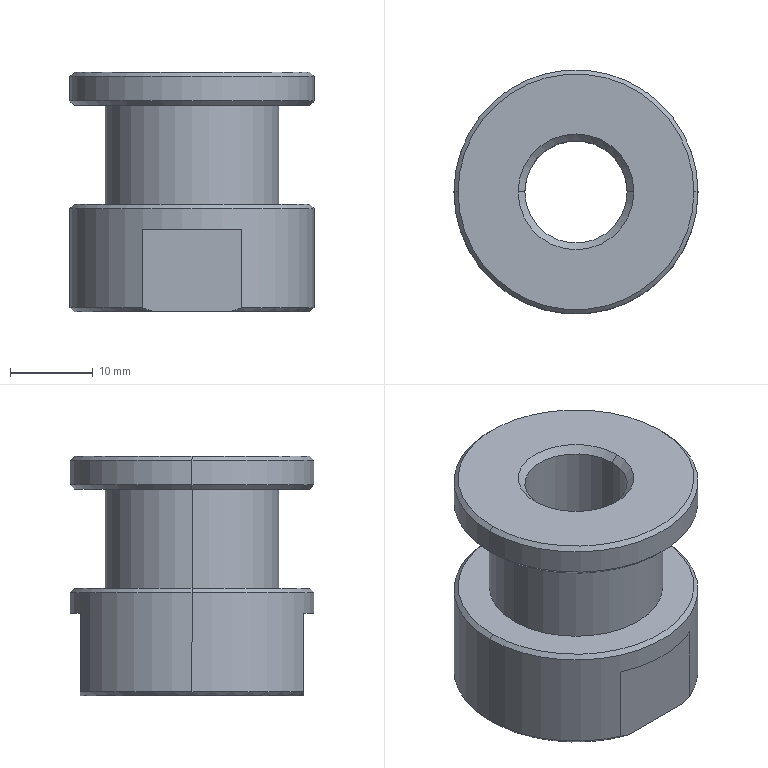Part | SolidWorks | features BaseBody 1 | 1 solid | 28 faces | box 29.5 x 29.5 x 29 mm | volume 12018 mm3 | cone 12 | cylinder 8 | plane 8 | commonest cylinder face diameters 29.5 x4 12.376 x2 21 x2
STEP:
#1=CARTESIAN_POINT('',(-6.188,0.,-28.188));
#2=VERTEX_POINT('',#1);
#3=CARTESIAN_POINT('',(6.188,0.,-28.188));
#4=VERTEX_POINT('',#3);
#5=CARTESIAN_POINT('',(0.,0.,-28.188));
#6=DIRECTION('',(0.,0.,1.));
#7=DIRECTION('',(1.,0.,0.));
#8=AXIS2_PLACEMENT_3D('',#5,#6,#7);
#9=CIRCLE('',#8,6.188);
#10=EDGE_CURVE('',#2,#4,#9,.T.);
#11=ORIENTED_EDGE('',*,*,#10,.F.);
#12=CARTESIAN_POINT('',(-6.188,0.,-0.812));
#13=VERTEX_POINT('',#12);
#14=CARTESIAN_POINT('',(-6.188,0.,-50.));
#15=DIRECTION('',(0.,0.,1.));
#16=VECTOR('',#15,1000.);
#17=LINE('',#14,#16);
#18=EDGE_CURVE('',#2,#13,#17,.T.);
#19=ORIENTED_EDGE('',*,*,#18,.T.);
#20=CARTESIAN_POINT('',(6.188,0.,-0.812));
#21=VERTEX_POINT('',#20);
#22=CARTESIAN_POINT('',(0.,0.,-0.812));
#23=DIRECTION('',(0.,0.,-1.));
#24=DIRECTION('',(1.,0.,0.));
#25=AXIS2_PLACEMENT_3D('',#22,#23,#24);
#26=CIRCLE('',#25,6.188);
#27=EDGE_CURVE('',#21,#13,#26,.T.);
#28=ORIENTED_EDGE('',*,*,#27,.F.);
#29=CARTESIAN_POINT('',(6.188,0.,-50.));
#30=DIRECTION('',(0.,0.,1.));
#31=VECTOR('',#30,1000.);
#32=LINE('',#29,#31);
#33=EDGE_CURVE('',#4,#21,#32,.T.);
#34=ORIENTED_EDGE('',*,*,#33,.F.);
#35=EDGE_LOOP('',(#11,#19,#28,#34));
#36=FACE_OUTER_BOUND('',#35,.T.);
#37=CARTESIAN_POINT('',(0.,0.,-50.));
#38=DIRECTION('',(0.,0.,1.));
#39=DIRECTION('',(1.,0.,0.));
#40=AXIS2_PLACEMENT_3D('',#37,#38,#39);
#41=CYLINDRICAL_SURFACE('',#40,6.188);
#42=ADVANCED_FACE('',(#36),#41,.F.);
#43=ORIENTED_EDGE('',*,*,#27,.T.);
#44=CARTESIAN_POINT('',(-7.,0.,0.));
#45=VERTEX_POINT('',#44);
#46=CARTESIAN_POINT('',(-7.,0.,0.));
#47=DIRECTION('',(-0.7071,0.,0.7071));
#48=VECTOR('',#47,1000.);
#49=LINE('',#46,#48);
#50=EDGE_CURVE('',#13,#45,#49,.T.);
#51=ORIENTED_EDGE('',*,*,#50,.T.);
#52=CARTESIAN_POINT('',(7.,0.,0.));
#53=VERTEX_POINT('',#52);
#54=CARTESIAN_POINT('',(0.,0.,0.));
#55=DIRECTION('',(0.,0.,-1.));
#56=DIRECTION('',(1.,0.,0.));
#57=AXIS2_PLACEMENT_3D('',#54,#55,#56);
#58=CIRCLE('',#57,7.);
#59=EDGE_CURVE('',#53,#45,#58,.T.);
#60=ORIENTED_EDGE('',*,*,#59,.F.);
#61=CARTESIAN_POINT('',(7.,0.,0.));
#62=DIRECTION('',(0.7071,0.,0.7071));
#63=VECTOR('',#62,1000.);
#64=LINE('',#61,#63);
#65=EDGE_CURVE('',#21,#53,#64,.T.);
#66=ORIENTED_EDGE('',*,*,#65,.F.);
#67=EDGE_LOOP('',(#43,#51,#60,#66));
#68=FACE_OUTER_BOUND('',#67,.T.);
#69=CARTESIAN_POINT('',(0.,0.,0.));
#70=DIRECTION('',(0.,0.,1.));
#71=DIRECTION('',(1.,0.,0.));
#72=AXIS2_PLACEMENT_3D('',#69,#70,#71);
#73=CONICAL_SURFACE('',#72,7.,0.7854);
#74=ADVANCED_FACE('',(#68),#73,.F.);
#75=ORIENTED_EDGE('',*,*,#10,.T.);
#76=CARTESIAN_POINT('',(7.,0.,-29.));
#77=VERTEX_POINT('',#76);
#78=CARTESIAN_POINT('',(7.,0.,-29.));
#79=DIRECTION('',(0.7071,0.,-0.7071));
#80=VECTOR('',#79,1000.);
#81=LINE('',#78,#80);
#82=EDGE_CURVE('',#4,#77,#81,.T.);
#83=ORIENTED_EDGE('',*,*,#82,.T.);
#84=CARTESIAN_POINT('',(-7.,0.,-29.));
#85=VERTEX_POINT('',#84);
#86=CARTESIAN_POINT('',(0.,0.,-29.));
#87=DIRECTION('',(0.,0.,1.));
#88=DIRECTION('',(-1.,0.,0.));
#89=AXIS2_PLACEMENT_3D('',#86,#87,#88);
#90=CIRCLE('',#89,7.);
#91=EDGE_CURVE('',#85,#77,#90,.T.);
#92=ORIENTED_EDGE('',*,*,#91,.F.);
#93=CARTESIAN_POINT('',(-7.,0.,-29.));
#94=DIRECTION('',(-0.7071,0.,-0.7071));
#95=VECTOR('',#94,1000.);
#96=LINE('',#93,#95);
#97=EDGE_CURVE('',#2,#85,#96,.T.);
#98=ORIENTED_EDGE('',*,*,#97,.F.);
#99=EDGE_LOOP('',(#75,#83,#92,#98));
#100=FACE_OUTER_BOUND('',#99,.T.);
#101=CARTESIAN_POINT('',(0.,0.,-29.));
#102=DIRECTION('',(0.,0.,-1.));
#103=DIRECTION('',(-1.,0.,0.));
#104=AXIS2_PLACEMENT_3D('',#101,#102,#103);
#105=CONICAL_SURFACE('',#104,7.,0.7854);
#106=ADVANCED_FACE('',(#100),#105,.F.);
#107=CARTESIAN_POINT('',(-14.25,0.,0.));
#108=VERTEX_POINT('',#107);
#109=CARTESIAN_POINT('',(14.25,0.,0.));
#110=VERTEX_POINT('',#109);
#111=CARTESIAN_POINT('',(0.,0.,0.));
#112=DIRECTION('',(0.,0.,-1.));
#113=DIRECTION('',(-1.,0.,0.));
#114=AXIS2_PLACEMENT_3D('',#111,#112,#113);
#115=CIRCLE('',#114,14.25);
#116=EDGE_CURVE('',#108,#110,#115,.T.);
#117=ORIENTED_EDGE('',*,*,#116,.T.);
#118=CARTESIAN_POINT('',(14.75,0.,-0.5));
#119=VERTEX_POINT('',#118);
#120=CARTESIAN_POINT('',(14.75,0.,-0.5));
#121=DIRECTION('',(0.7071,0.,-0.7071));
#122=VECTOR('',#121,1000.);
#123=LINE('',#120,#122);
#124=EDGE_CURVE('',#110,#119,#123,.T.);
#125=ORIENTED_EDGE('',*,*,#124,.T.);
#126=CARTESIAN_POINT('',(-14.75,0.,-0.5));
#127=VERTEX_POINT('',#126);
#128=CARTESIAN_POINT('',(0.,0.,-0.5));
#129=DIRECTION('',(0.,0.,1.));
#130=DIRECTION('',(-1.,0.,0.));
#131=AXIS2_PLACEMENT_3D('',#128,#129,#130);
#132=CIRCLE('',#131,14.75);
#133=EDGE_CURVE('',#119,#127,#132,.T.);
#134=ORIENTED_EDGE('',*,*,#133,.T.);
#135=CARTESIAN_POINT('',(-14.75,0.,-0.5));
#136=DIRECTION('',(-0.7071,0.,-0.7071));
#137=VECTOR('',#136,1000.);
#138=LINE('',#135,#137);
#139=EDGE_CURVE('',#108,#127,#138,.T.);
#140=ORIENTED_EDGE('',*,*,#139,.F.);
#141=EDGE_LOOP('',(#117,#125,#134,#140));
#142=FACE_OUTER_BOUND('',#141,.T.);
#143=CARTESIAN_POINT('',(0.,0.,-0.5));
#144=DIRECTION('',(0.,0.,-1.));
#145=DIRECTION('',(-1.,0.,0.));
#146=AXIS2_PLACEMENT_3D('',#143,#144,#145);
#147=CONICAL_SURFACE('',#146,14.75,0.7854);
#148=ADVANCED_FACE('',(#142),#147,.T.);
#149=CARTESIAN_POINT('',(14.75,0.,-3.5));
#150=VERTEX_POINT('',#149);
#151=CARTESIAN_POINT('',(-14.75,0.,-3.5));
#152=VERTEX_POINT('',#151);
#153=CARTESIAN_POINT('',(0.,0.,-3.5));
#154=DIRECTION('',(0.,0.,1.));
#155=DIRECTION('',(1.,0.,0.));
#156=AXIS2_PLACEMENT_3D('',#153,#154,#155);
#157=CIRCLE('',#156,14.75);
#158=EDGE_CURVE('',#150,#152,#157,.T.);
#159=ORIENTED_EDGE('',*,*,#158,.T.);
#160=CARTESIAN_POINT('',(-14.75,0.,-50.));
#161=DIRECTION('',(0.,0.,1.));
#162=VECTOR('',#161,1000.);
#163=LINE('',#160,#162);
#164=EDGE_CURVE('',#152,#127,#163,.T.);
#165=ORIENTED_EDGE('',*,*,#164,.T.);
#166=ORIENTED_EDGE('',*,*,#133,.F.);
#167=CARTESIAN_POINT('',(14.75,0.,-50.));
#168=DIRECTION('',(0.,0.,1.));
#169=VECTOR('',#168,1000.);
#170=LINE('',#167,#169);
#171=EDGE_CURVE('',#150,#119,#170,.T.);
#172=ORIENTED_EDGE('',*,*,#171,.F.);
#173=EDGE_LOOP('',(#159,#165,#166,#172));
#174=FACE_OUTER_BOUND('',#173,.T.);
#175=CARTESIAN_POINT('',(0.,0.,-50.));
#176=DIRECTION('',(0.,0.,1.));
#177=DIRECTION('',(1.,0.,0.));
#178=AXIS2_PLACEMENT_3D('',#175,#176,#177);
#179=CYLINDRICAL_SURFACE('',#178,14.75);
#180=ADVANCED_FACE('',(#174),#179,.T.);
#181=CARTESIAN_POINT('',(-14.75,0.,-28.5));
#182=VERTEX_POINT('',#181);
#183=CARTESIAN_POINT('',(-5.942,13.5,-28.5));
#184=VERTEX_POINT('',#183);
#185=CARTESIAN_POINT('',(0.,0.,-28.5));
#186=DIRECTION('',(0.,0.,-1.));
#187=DIRECTION('',(1.,0.,0.));
#188=AXIS2_PLACEMENT_3D('',#185,#186,#187);
#189=CIRCLE('',#188,14.75);
#190=EDGE_CURVE('',#182,#184,#189,.T.);
#191=ORIENTED_EDGE('',*,*,#190,.F.);
#192=CARTESIAN_POINT('',(-14.75,0.,-16.5));
#193=VERTEX_POINT('',#192);
#194=CARTESIAN_POINT('',(-14.75,0.,-50.));
#195=DIRECTION('',(0.,0.,1.));
#196=VECTOR('',#195,1000.);
#197=LINE('',#194,#196);
#198=EDGE_CURVE('',#182,#193,#197,.T.);
#199=ORIENTED_EDGE('',*,*,#198,.T.);
#200=CARTESIAN_POINT('',(14.75,0.,-16.5));
#201=VERTEX_POINT('',#200);
#202=CARTESIAN_POINT('',(0.,0.,-16.5));
#203=DIRECTION('',(0.,0.,-1.));
#204=DIRECTION('',(1.,0.,0.));
#205=AXIS2_PLACEMENT_3D('',#202,#203,#204);
#206=CIRCLE('',#205,14.75);
#207=EDGE_CURVE('',#193,#201,#206,.T.);
#208=ORIENTED_EDGE('',*,*,#207,.T.);
#209=CARTESIAN_POINT('',(14.75,0.,-28.5));
#210=VERTEX_POINT('',#209);
#211=CARTESIAN_POINT('',(14.75,0.,-50.));
#212=DIRECTION('',(0.,0.,1.));
#213=VECTOR('',#212,1000.);
#214=LINE('',#211,#213);
#215=EDGE_CURVE('',#210,#201,#214,.T.);
#216=ORIENTED_EDGE('',*,*,#215,.F.);
#217=CARTESIAN_POINT('',(5.942,13.5,-28.5));
#218=VERTEX_POINT('',#217);
#219=CARTESIAN_POINT('',(0.,0.,-28.5));
#220=DIRECTION('',(0.,0.,-1.));
#221=DIRECTION('',(1.,0.,0.));
#222=AXIS2_PLACEMENT_3D('',#219,#220,#221);
#223=CIRCLE('',#222,14.75);
#224=EDGE_CURVE('',#218,#210,#223,.T.);
#225=ORIENTED_EDGE('',*,*,#224,.F.);
#226=CARTESIAN_POINT('',(5.942,13.5,-19.));
#227=VERTEX_POINT('',#226);
#228=CARTESIAN_POINT('',(5.942,13.5,-19.));
#229=DIRECTION('',(0.,0.,1.));
#230=VECTOR('',#229,1000.);
#231=LINE('',#228,#230);
#232=EDGE_CURVE('',#218,#227,#231,.T.);
#233=ORIENTED_EDGE('',*,*,#232,.T.);
#234=CARTESIAN_POINT('',(-5.942,13.5,-19.));
#235=VERTEX_POINT('',#234);
#236=CARTESIAN_POINT('',(0.,0.,-19.));
#237=DIRECTION('',(0.,0.,1.));
#238=DIRECTION('',(1.,0.,0.));
#239=AXIS2_PLACEMENT_3D('',#236,#237,#238);
#240=CIRCLE('',#239,14.75);
#241=EDGE_CURVE('',#227,#235,#240,.T.);
#242=ORIENTED_EDGE('',*,*,#241,.T.);
#243=CARTESIAN_POINT('',(-5.942,13.5,-19.));
#244=DIRECTION('',(0.,0.,-1.));
#245=VECTOR('',#244,1000.);
#246=LINE('',#243,#245);
#247=EDGE_CURVE('',#235,#184,#246,.T.);
#248=ORIENTED_EDGE('',*,*,#247,.T.);
#249=EDGE_LOOP('',(#191,#199,#208,#216,#225,#233,#242,#248));
#250=FACE_OUTER_BOUND('',#249,.T.);
#251=CARTESIAN_POINT('',(0.,0.,-50.));
#252=DIRECTION('',(0.,0.,1.));
#253=DIRECTION('',(1.,0.,0.));
#254=AXIS2_PLACEMENT_3D('',#251,#252,#253);
#255=CYLINDRICAL_SURFACE('',#254,14.75);
#256=ADVANCED_FACE('',(#250),#255,.T.);
#257=CARTESIAN_POINT('',(14.25,0.,-4.));
#258=VERTEX_POINT('',#257);
#259=CARTESIAN_POINT('',(-14.25,0.,-4.));
#260=VERTEX_POINT('',#259);
#261=CARTESIAN_POINT('',(0.,0.,-4.));
#262=DIRECTION('',(0.,0.,1.));
#263=DIRECTION('',(1.,0.,0.));
#264=AXIS2_PLACEMENT_3D('',#261,#262,#263);
#265=CIRCLE('',#264,14.25);
#266=EDGE_CURVE('',#258,#260,#265,.T.);
#267=ORIENTED_EDGE('',*,*,#266,.T.);
#268=CARTESIAN_POINT('',(-14.75,0.,-3.5));
#269=DIRECTION('',(-0.7071,0.,0.7071));
#270=VECTOR('',#269,1000.);
#271=LINE('',#268,#270);
#272=EDGE_CURVE('',#260,#152,#271,.T.);
#273=ORIENTED_EDGE('',*,*,#272,.T.);
#274=ORIENTED_EDGE('',*,*,#158,.F.);
#275=CARTESIAN_POINT('',(14.75,0.,-3.5));
#276=DIRECTION('',(0.7071,0.,0.7071));
#277=VECTOR('',#276,1000.);
#278=LINE('',#275,#277);
#279=EDGE_CURVE('',#258,#150,#278,.T.);
#280=ORIENTED_EDGE('',*,*,#279,.F.);
#281=EDGE_LOOP('',(#267,#273,#274,#280));
#282=FACE_OUTER_BOUND('',#281,.T.);
#283=CARTESIAN_POINT('',(0.,0.,-3.5));
#284=DIRECTION('',(0.,0.,1.));
#285=DIRECTION('',(1.,0.,0.));
#286=AXIS2_PLACEMENT_3D('',#283,#284,#285);
#287=CONICAL_SURFACE('',#286,14.75,0.7854);
#288=ADVANCED_FACE('',(#282),#287,.T.);
#289=CARTESIAN_POINT('',(-14.25,0.,-16.));
#290=VERTEX_POINT('',#289);
#291=CARTESIAN_POINT('',(14.25,0.,-16.));
#292=VERTEX_POINT('',#291);
#293=CARTESIAN_POINT('',(0.,0.,-16.));
#294=DIRECTION('',(0.,0.,-1.));
#295=DIRECTION('',(-1.,0.,0.));
#296=AXIS2_PLACEMENT_3D('',#293,#294,#295);
#297=CIRCLE('',#296,14.25);
#298=EDGE_CURVE('',#290,#292,#297,.T.);
#299=ORIENTED_EDGE('',*,*,#298,.T.);
#300=CARTESIAN_POINT('',(14.75,0.,-16.5));
#301=DIRECTION('',(0.7071,0.,-0.7071));
#302=VECTOR('',#301,1000.);
#303=LINE('',#300,#302);
#304=EDGE_CURVE('',#292,#201,#303,.T.);
#305=ORIENTED_EDGE('',*,*,#304,.T.);
#306=ORIENTED_EDGE('',*,*,#207,.F.);
#307=CARTESIAN_POINT('',(-14.75,0.,-16.5));
#308=DIRECTION('',(-0.7071,0.,-0.7071));
#309=VECTOR('',#308,1000.);
#310=LINE('',#307,#309);
#311=EDGE_CURVE('',#290,#193,#310,.T.);
#312=ORIENTED_EDGE('',*,*,#311,.F.);
#313=EDGE_LOOP('',(#299,#305,#306,#312));
#314=FACE_OUTER_BOUND('',#313,.T.);
#315=CARTESIAN_POINT('',(0.,0.,-16.5));
#316=DIRECTION('',(0.,0.,-1.));
#317=DIRECTION('',(-1.,0.,0.));
#318=AXIS2_PLACEMENT_3D('',#315,#316,#317);
#319=CONICAL_SURFACE('',#318,14.75,0.7854);
#320=ADVANCED_FACE('',(#314),#319,.T.);
#321=CARTESIAN_POINT('',(10.5,0.,-16.));
#322=VERTEX_POINT('',#321);
#323=CARTESIAN_POINT('',(-10.5,0.,-16.));
#324=VERTEX_POINT('',#323);
#325=CARTESIAN_POINT('',(0.,0.,-16.));
#326=DIRECTION('',(0.,0.,1.));
#327=DIRECTION('',(1.,0.,0.));
#328=AXIS2_PLACEMENT_3D('',#325,#326,#327);
#329=CIRCLE('',#328,10.5);
#330=EDGE_CURVE('',#322,#324,#329,.T.);
#331=ORIENTED_EDGE('',*,*,#330,.T.);
#332=CARTESIAN_POINT('',(-10.5,0.,-4.));
#333=VERTEX_POINT('',#332);
#334=CARTESIAN_POINT('',(-10.5,0.,-50.));
#335=DIRECTION('',(0.,0.,1.));
#336=VECTOR('',#335,1000.);
#337=LINE('',#334,#336);
#338=EDGE_CURVE('',#324,#333,#337,.T.);
#339=ORIENTED_EDGE('',*,*,#338,.T.);
#340=CARTESIAN_POINT('',(10.5,0.,-4.));
#341=VERTEX_POINT('',#340);
#342=CARTESIAN_POINT('',(0.,0.,-4.));
#343=DIRECTION('',(0.,0.,-1.));
#344=DIRECTION('',(1.,0.,0.));
#345=AXIS2_PLACEMENT_3D('',#342,#343,#344);
#346=CIRCLE('',#345,10.5);
#347=EDGE_CURVE('',#333,#341,#346,.T.);
#348=ORIENTED_EDGE('',*,*,#347,.T.);
#349=CARTESIAN_POINT('',(10.5,0.,-50.));
#350=DIRECTION('',(0.,0.,1.));
#351=VECTOR('',#350,1000.);
#352=LINE('',#349,#351);
#353=EDGE_CURVE('',#322,#341,#352,.T.);
#354=ORIENTED_EDGE('',*,*,#353,.F.);
#355=EDGE_LOOP('',(#331,#339,#348,#354));
#356=FACE_OUTER_BOUND('',#355,.T.);
#357=CARTESIAN_POINT('',(0.,0.,-50.));
#358=DIRECTION('',(0.,0.,1.));
#359=DIRECTION('',(1.,0.,0.));
#360=AXIS2_PLACEMENT_3D('',#357,#358,#359);
#361=CYLINDRICAL_SURFACE('',#360,10.5);
#362=ADVANCED_FACE('',(#356),#361,.T.);
#363=ORIENTED_EDGE('',*,*,#18,.F.);
#364=CARTESIAN_POINT('',(0.,0.,-28.188));
#365=DIRECTION('',(0.,0.,1.));
#366=DIRECTION('',(1.,0.,0.));
#367=AXIS2_PLACEMENT_3D('',#364,#365,#366);
#368=CIRCLE('',#367,6.188);
#369=EDGE_CURVE('',#4,#2,#368,.T.);
#370=ORIENTED_EDGE('',*,*,#369,.F.);
#371=ORIENTED_EDGE('',*,*,#33,.T.);
#372=CARTESIAN_POINT('',(0.,0.,-0.812));
#373=DIRECTION('',(0.,0.,-1.));
#374=DIRECTION('',(1.,0.,0.));
#375=AXIS2_PLACEMENT_3D('',#372,#373,#374);
#376=CIRCLE('',#375,6.188);
#377=EDGE_CURVE('',#13,#21,#376,.T.);
#378=ORIENTED_EDGE('',*,*,#377,.F.);
#379=EDGE_LOOP('',(#363,#370,#371,#378));
#380=FACE_OUTER_BOUND('',#379,.T.);
#381=CARTESIAN_POINT('',(0.,0.,-50.));
#382=DIRECTION('',(0.,0.,1.));
#383=DIRECTION('',(1.,0.,0.));
#384=AXIS2_PLACEMENT_3D('',#381,#382,#383);
#385=CYLINDRICAL_SURFACE('',#384,6.188);
#386=ADVANCED_FACE('',(#380),#385,.F.);
#387=ORIENTED_EDGE('',*,*,#50,.F.);
#388=ORIENTED_EDGE('',*,*,#377,.T.);
#389=ORIENTED_EDGE('',*,*,#65,.T.);
#390=CARTESIAN_POINT('',(0.,0.,0.));
#391=DIRECTION('',(0.,0.,-1.));
#392=DIRECTION('',(1.,0.,0.));
#393=AXIS2_PLACEMENT_3D('',#390,#391,#392);
#394=CIRCLE('',#393,7.);
#395=EDGE_CURVE('',#45,#53,#394,.T.);
#396=ORIENTED_EDGE('',*,*,#395,.F.);
#397=EDGE_LOOP('',(#387,#388,#389,#396));
#398=FACE_OUTER_BOUND('',#397,.T.);
#399=CARTESIAN_POINT('',(0.,0.,0.));
#400=DIRECTION('',(0.,0.,1.));
#401=DIRECTION('',(1.,0.,0.));
#402=AXIS2_PLACEMENT_3D('',#399,#400,#401);
#403=CONICAL_SURFACE('',#402,7.,0.7854);
#404=ADVANCED_FACE('',(#398),#403,.F.);
#405=ORIENTED_EDGE('',*,*,#82,.F.);
#406=ORIENTED_EDGE('',*,*,#369,.T.);
#407=ORIENTED_EDGE('',*,*,#97,.T.);
#408=CARTESIAN_POINT('',(0.,0.,-29.));
#409=DIRECTION('',(0.,0.,1.));
#410=DIRECTION('',(-1.,0.,0.));
#411=AXIS2_PLACEMENT_3D('',#408,#409,#410);
#412=CIRCLE('',#411,7.);
#413=EDGE_CURVE('',#77,#85,#412,.T.);
#414=ORIENTED_EDGE('',*,*,#413,.F.);
#415=EDGE_LOOP('',(#405,#406,#407,#414));
#416=FACE_OUTER_BOUND('',#415,.T.);
#417=CARTESIAN_POINT('',(0.,0.,-29.));
#418=DIRECTION('',(0.,0.,-1.));
#419=DIRECTION('',(-1.,0.,0.));
#420=AXIS2_PLACEMENT_3D('',#417,#418,#419);
#421=CONICAL_SURFACE('',#420,7.,0.7854);
#422=ADVANCED_FACE('',(#416),#421,.F.);
#423=ORIENTED_EDGE('',*,*,#59,.T.);
#424=ORIENTED_EDGE('',*,*,#395,.T.);
#425=EDGE_LOOP('',(#423,#424));
#426=FACE_BOUND('',#425,.T.);
#427=ORIENTED_EDGE('',*,*,#116,.F.);
#428=CARTESIAN_POINT('',(0.,0.,0.));
#429=DIRECTION('',(0.,0.,-1.));
#430=DIRECTION('',(-1.,0.,0.));
#431=AXIS2_PLACEMENT_3D('',#428,#429,#430);
#432=CIRCLE('',#431,14.25);
#433=EDGE_CURVE('',#110,#108,#432,.T.);
#434=ORIENTED_EDGE('',*,*,#433,.F.);
#435=EDGE_LOOP('',(#427,#434));
#436=FACE_OUTER_BOUND('',#435,.T.);
#437=CARTESIAN_POINT('',(0.,0.,0.));
#438=DIRECTION('',(0.,0.,-1.));
#439=DIRECTION('',(-1.,0.,0.));
#440=AXIS2_PLACEMENT_3D('',#437,#438,#439);
#441=PLANE('',#440);
#442=ADVANCED_FACE('',(#426,#436),#441,.F.);
#443=CARTESIAN_POINT('',(4.562,13.5,-29.));
#444=VERTEX_POINT('',#443);
#445=CARTESIAN_POINT('',(-4.562,13.5,-29.));
#446=VERTEX_POINT('',#445);
#447=CARTESIAN_POINT('',(0.,13.5,-29.));
#448=DIRECTION('',(-1.,0.,0.));
#449=VECTOR('',#448,1000.);
#450=LINE('',#447,#449);
#451=EDGE_CURVE('',#444,#446,#450,.T.);
#452=ORIENTED_EDGE('',*,*,#451,.F.);
#453=CARTESIAN_POINT('',(4.562,-13.5,-29.));
#454=VERTEX_POINT('',#453);
#455=CARTESIAN_POINT('',(0.,0.,-29.));
#456=DIRECTION('',(0.,0.,1.));
#457=DIRECTION('',(0.,-1.,0.));
#458=AXIS2_PLACEMENT_3D('',#455,#456,#457);
#459=CIRCLE('',#458,14.25);
#460=EDGE_CURVE('',#454,#444,#459,.T.);
#461=ORIENTED_EDGE('',*,*,#460,.F.);
#462=CARTESIAN_POINT('',(-4.562,-13.5,-29.));
#463=VERTEX_POINT('',#462);
#464=CARTESIAN_POINT('',(0.,-13.5,-29.));
#465=DIRECTION('',(1.,0.,0.));
#466=VECTOR('',#465,1000.);
#467=LINE('',#464,#466);
#468=EDGE_CURVE('',#463,#454,#467,.T.);
#469=ORIENTED_EDGE('',*,*,#468,.F.);
#470=CARTESIAN_POINT('',(0.,0.,-29.));
#471=DIRECTION('',(0.,0.,1.));
#472=DIRECTION('',(0.,-1.,0.));
#473=AXIS2_PLACEMENT_3D('',#470,#471,#472);
#474=CIRCLE('',#473,14.25);
#475=EDGE_CURVE('',#446,#463,#474,.T.);
#476=ORIENTED_EDGE('',*,*,#475,.F.);
#477=EDGE_LOOP('',(#452,#461,#469,#476));
#478=FACE_OUTER_BOUND('',#477,.T.);
#479=ORIENTED_EDGE('',*,*,#91,.T.);
#480=ORIENTED_EDGE('',*,*,#413,.T.);
#481=EDGE_LOOP('',(#479,#480));
#482=FACE_BOUND('',#481,.T.);
#483=CARTESIAN_POINT('',(0.,14.25,-29.));
#484=DIRECTION('',(0.,0.,1.));
#485=DIRECTION('',(1.,0.,0.));
#486=AXIS2_PLACEMENT_3D('',#483,#484,#485);
#487=PLANE('',#486);
#488=ADVANCED_FACE('',(#478,#482),#487,.F.);
#489=ORIENTED_EDGE('',*,*,#124,.F.);
#490=ORIENTED_EDGE('',*,*,#433,.T.);
#491=ORIENTED_EDGE('',*,*,#139,.T.);
#492=CARTESIAN_POINT('',(0.,0.,-0.5));
#493=DIRECTION('',(0.,0.,1.));
#494=DIRECTION('',(-1.,0.,0.));
#495=AXIS2_PLACEMENT_3D('',#492,#493,#494);
#496=CIRCLE('',#495,14.75);
#497=EDGE_CURVE('',#127,#119,#496,.T.);
#498=ORIENTED_EDGE('',*,*,#497,.T.);
#499=EDGE_LOOP('',(#489,#490,#491,#498));
#500=FACE_OUTER_BOUND('',#499,.T.);
#501=CARTESIAN_POINT('',(0.,0.,-0.5));
#502=DIRECTION('',(0.,0.,-1.));
#503=DIRECTION('',(-1.,0.,0.));
#504=AXIS2_PLACEMENT_3D('',#501,#502,#503);
#505=CONICAL_SURFACE('',#504,14.75,0.7854);
#506=ADVANCED_FACE('',(#500),#505,.T.);
#507=CARTESIAN_POINT('',(-5.942,-13.5,-28.5));
#508=VERTEX_POINT('',#507);
#509=CARTESIAN_POINT('',(0.,0.,-28.5));
#510=DIRECTION('',(0.,0.,-1.));
#511=DIRECTION('',(1.,0.,0.));
#512=AXIS2_PLACEMENT_3D('',#509,#510,#511);
#513=CIRCLE('',#512,14.75);
#514=EDGE_CURVE('',#508,#182,#513,.T.);
#515=ORIENTED_EDGE('',*,*,#514,.T.);
#516=ORIENTED_EDGE('',*,*,#190,.T.);
#517=CARTESIAN_POINT('',(-5.942,13.5,-28.5));
#518=CARTESIAN_POINT('',(-5.488,13.5,-28.683));
#519=CARTESIAN_POINT('',(-5.028,13.5,-28.851));
#520=CARTESIAN_POINT('',(-4.562,13.5,-29.));
#521=B_SPLINE_CURVE_WITH_KNOTS('',3,(#517,#518,#519,#520),.UNSPECIFIED.,.F.,.F.,(4,4),(0.,0.001468),.UNSPECIFIED.);
#522=EDGE_CURVE('',#184,#446,#521,.T.);
#523=ORIENTED_EDGE('',*,*,#522,.T.);
#524=ORIENTED_EDGE('',*,*,#475,.T.);
#525=CARTESIAN_POINT('',(-4.562,-13.5,-29.));
#526=CARTESIAN_POINT('',(-5.028,-13.5,-28.851));
#527=CARTESIAN_POINT('',(-5.488,-13.5,-28.683));
#528=CARTESIAN_POINT('',(-5.942,-13.5,-28.5));
#529=B_SPLINE_CURVE_WITH_KNOTS('',3,(#525,#526,#527,#528),.UNSPECIFIED.,.F.,.F.,(4,4),(0.,0.001468),.UNSPECIFIED.);
#530=EDGE_CURVE('',#463,#508,#529,.T.);
#531=ORIENTED_EDGE('',*,*,#530,.T.);
#532=EDGE_LOOP('',(#515,#516,#523,#524,#531));
#533=FACE_OUTER_BOUND('',#532,.T.);
#534=CARTESIAN_POINT('',(0.,0.,-28.5));
#535=DIRECTION('',(0.,0.,1.));
#536=DIRECTION('',(0.,-1.,0.));
#537=AXIS2_PLACEMENT_3D('',#534,#535,#536);
#538=CONICAL_SURFACE('',#537,14.75,0.7854);
#539=ADVANCED_FACE('',(#533),#538,.T.);
#540=CARTESIAN_POINT('',(5.942,13.5,-19.));
#541=DIRECTION('',(-1.,0.,0.));
#542=VECTOR('',#541,1000.);
#543=LINE('',#540,#542);
#544=EDGE_CURVE('',#227,#235,#543,.T.);
#545=ORIENTED_EDGE('',*,*,#544,.F.);
#546=ORIENTED_EDGE('',*,*,#232,.F.);
#547=CARTESIAN_POINT('',(4.562,13.5,-29.));
#548=CARTESIAN_POINT('',(5.028,13.5,-28.851));
#549=CARTESIAN_POINT('',(5.488,13.5,-28.683));
#550=CARTESIAN_POINT('',(5.942,13.5,-28.5));
#551=B_SPLINE_CURVE_WITH_KNOTS('',3,(#547,#548,#549,#550),.UNSPECIFIED.,.F.,.F.,(4,4),(0.,0.001468),.UNSPECIFIED.);
#552=EDGE_CURVE('',#444,#218,#551,.T.);
#553=ORIENTED_EDGE('',*,*,#552,.F.);
#554=ORIENTED_EDGE('',*,*,#451,.T.);
#555=ORIENTED_EDGE('',*,*,#522,.F.);
#556=ORIENTED_EDGE('',*,*,#247,.F.);
#557=EDGE_LOOP('',(#545,#546,#553,#554,#555,#556));
#558=FACE_OUTER_BOUND('',#557,.T.);
#559=CARTESIAN_POINT('',(5.942,13.5,-19.));
#560=DIRECTION('',(0.,-1.,0.));
#561=DIRECTION('',(0.,0.,-1.));
#562=AXIS2_PLACEMENT_3D('',#559,#560,#561);
#563=PLANE('',#562);
#564=ADVANCED_FACE('',(#558),#563,.F.);
#565=ORIENTED_EDGE('',*,*,#460,.T.);
#566=ORIENTED_EDGE('',*,*,#552,.T.);
#567=ORIENTED_EDGE('',*,*,#224,.T.);
#568=CARTESIAN_POINT('',(5.942,-13.5,-28.5));
#569=VERTEX_POINT('',#568);
#570=CARTESIAN_POINT('',(0.,0.,-28.5));
#571=DIRECTION('',(0.,0.,-1.));
#572=DIRECTION('',(1.,0.,0.));
#573=AXIS2_PLACEMENT_3D('',#570,#571,#572);
#574=CIRCLE('',#573,14.75);
#575=EDGE_CURVE('',#210,#569,#574,.T.);
#576=ORIENTED_EDGE('',*,*,#575,.T.);
#577=CARTESIAN_POINT('',(5.942,-13.5,-28.5));
#578=CARTESIAN_POINT('',(5.488,-13.5,-28.683));
#579=CARTESIAN_POINT('',(5.028,-13.5,-28.851));
#580=CARTESIAN_POINT('',(4.562,-13.5,-29.));
#581=B_SPLINE_CURVE_WITH_KNOTS('',3,(#577,#578,#579,#580),.UNSPECIFIED.,.F.,.F.,(4,4),(0.,0.001468),.UNSPECIFIED.);
#582=EDGE_CURVE('',#569,#454,#581,.T.);
#583=ORIENTED_EDGE('',*,*,#582,.T.);
#584=EDGE_LOOP('',(#565,#566,#567,#576,#583));
#585=FACE_OUTER_BOUND('',#584,.T.);
#586=CARTESIAN_POINT('',(0.,0.,-28.5));
#587=DIRECTION('',(0.,0.,1.));
#588=DIRECTION('',(0.,-1.,0.));
#589=AXIS2_PLACEMENT_3D('',#586,#587,#588);
#590=CONICAL_SURFACE('',#589,14.75,0.7854);
#591=ADVANCED_FACE('',(#585),#590,.T.);
#592=CARTESIAN_POINT('',(-5.942,-13.5,-19.));
#593=VERTEX_POINT('',#592);
#594=CARTESIAN_POINT('',(5.942,-13.5,-19.));
#595=VERTEX_POINT('',#594);
#596=CARTESIAN_POINT('',(-5.942,-13.5,-19.));
#597=DIRECTION('',(1.,0.,0.));
#598=VECTOR('',#597,1000.);
#599=LINE('',#596,#598);
#600=EDGE_CURVE('',#593,#595,#599,.T.);
#601=ORIENTED_EDGE('',*,*,#600,.F.);
#602=CARTESIAN_POINT('',(-5.942,-13.5,-19.));
#603=DIRECTION('',(0.,0.,1.));
#604=VECTOR('',#603,1000.);
#605=LINE('',#602,#604);
#606=EDGE_CURVE('',#508,#593,#605,.T.);
#607=ORIENTED_EDGE('',*,*,#606,.F.);
#608=ORIENTED_EDGE('',*,*,#530,.F.);
#609=ORIENTED_EDGE('',*,*,#468,.T.);
#610=ORIENTED_EDGE('',*,*,#582,.F.);
#611=CARTESIAN_POINT('',(5.942,-13.5,-19.));
#612=DIRECTION('',(0.,0.,-1.));
#613=VECTOR('',#612,1000.);
#614=LINE('',#611,#613);
#615=EDGE_CURVE('',#595,#569,#614,.T.);
#616=ORIENTED_EDGE('',*,*,#615,.F.);
#617=EDGE_LOOP('',(#601,#607,#608,#609,#610,#616));
#618=FACE_OUTER_BOUND('',#617,.T.);
#619=CARTESIAN_POINT('',(-5.942,-13.5,-19.));
#620=DIRECTION('',(0.,1.,0.));
#621=DIRECTION('',(0.,0.,1.));
#622=AXIS2_PLACEMENT_3D('',#619,#620,#621);
#623=PLANE('',#622);
#624=ADVANCED_FACE('',(#618),#623,.F.);
#625=ORIENTED_EDGE('',*,*,#164,.F.);
#626=CARTESIAN_POINT('',(0.,0.,-3.5));
#627=DIRECTION('',(0.,0.,1.));
#628=DIRECTION('',(1.,0.,0.));
#629=AXIS2_PLACEMENT_3D('',#626,#627,#628);
#630=CIRCLE('',#629,14.75);
#631=EDGE_CURVE('',#152,#150,#630,.T.);
#632=ORIENTED_EDGE('',*,*,#631,.T.);
#633=ORIENTED_EDGE('',*,*,#171,.T.);
#634=ORIENTED_EDGE('',*,*,#497,.F.);
#635=EDGE_LOOP('',(#625,#632,#633,#634));
#636=FACE_OUTER_BOUND('',#635,.T.);
#637=CARTESIAN_POINT('',(0.,0.,-50.));
#638=DIRECTION('',(0.,0.,1.));
#639=DIRECTION('',(1.,0.,0.));
#640=AXIS2_PLACEMENT_3D('',#637,#638,#639);
#641=CYLINDRICAL_SURFACE('',#640,14.75);
#642=ADVANCED_FACE('',(#636),#641,.T.);
#643=ORIENTED_EDGE('',*,*,#198,.F.);
#644=ORIENTED_EDGE('',*,*,#514,.F.);
#645=ORIENTED_EDGE('',*,*,#606,.T.);
#646=CARTESIAN_POINT('',(0.,0.,-19.));
#647=DIRECTION('',(0.,0.,1.));
#648=DIRECTION('',(1.,0.,0.));
#649=AXIS2_PLACEMENT_3D('',#646,#647,#648);
#650=CIRCLE('',#649,14.75);
#651=EDGE_CURVE('',#593,#595,#650,.T.);
#652=ORIENTED_EDGE('',*,*,#651,.T.);
#653=ORIENTED_EDGE('',*,*,#615,.T.);
#654=ORIENTED_EDGE('',*,*,#575,.F.);
#655=ORIENTED_EDGE('',*,*,#215,.T.);
#656=CARTESIAN_POINT('',(0.,0.,-16.5));
#657=DIRECTION('',(0.,0.,-1.));
#658=DIRECTION('',(1.,0.,0.));
#659=AXIS2_PLACEMENT_3D('',#656,#657,#658);
#660=CIRCLE('',#659,14.75);
#661=EDGE_CURVE('',#201,#193,#660,.T.);
#662=ORIENTED_EDGE('',*,*,#661,.T.);
#663=EDGE_LOOP('',(#643,#644,#645,#652,#653,#654,#655,#662));
#664=FACE_OUTER_BOUND('',#663,.T.);
#665=CARTESIAN_POINT('',(0.,0.,-50.));
#666=DIRECTION('',(0.,0.,1.));
#667=DIRECTION('',(1.,0.,0.));
#668=AXIS2_PLACEMENT_3D('',#665,#666,#667);
#669=CYLINDRICAL_SURFACE('',#668,14.75);
#670=ADVANCED_FACE('',(#664),#669,.T.);
#671=ORIENTED_EDGE('',*,*,#544,.T.);
#672=ORIENTED_EDGE('',*,*,#241,.F.);
#673=EDGE_LOOP('',(#671,#672));
#674=FACE_OUTER_BOUND('',#673,.T.);
#675=CARTESIAN_POINT('',(0.,0.,-19.));
#676=DIRECTION('',(0.,0.,-1.));
#677=DIRECTION('',(-1.,0.,0.));
#678=AXIS2_PLACEMENT_3D('',#675,#676,#677);
#679=PLANE('',#678);
#680=ADVANCED_FACE('',(#674),#679,.T.);
#681=ORIENTED_EDGE('',*,*,#600,.T.);
#682=ORIENTED_EDGE('',*,*,#651,.F.);
#683=EDGE_LOOP('',(#681,#682));
#684=FACE_OUTER_BOUND('',#683,.T.);
#685=CARTESIAN_POINT('',(0.,0.,-19.));
#686=DIRECTION('',(0.,0.,-1.));
#687=DIRECTION('',(-1.,0.,0.));
#688=AXIS2_PLACEMENT_3D('',#685,#686,#687);
#689=PLANE('',#688);
#690=ADVANCED_FACE('',(#684),#689,.T.);
#691=ORIENTED_EDGE('',*,*,#272,.F.);
#692=CARTESIAN_POINT('',(0.,0.,-4.));
#693=DIRECTION('',(0.,0.,1.));
#694=DIRECTION('',(1.,0.,0.));
#695=AXIS2_PLACEMENT_3D('',#692,#693,#694);
#696=CIRCLE('',#695,14.25);
#697=EDGE_CURVE('',#260,#258,#696,.T.);
#698=ORIENTED_EDGE('',*,*,#697,.T.);
#699=ORIENTED_EDGE('',*,*,#279,.T.);
#700=ORIENTED_EDGE('',*,*,#631,.F.);
#701=EDGE_LOOP('',(#691,#698,#699,#700));
#702=FACE_OUTER_BOUND('',#701,.T.);
#703=CARTESIAN_POINT('',(0.,0.,-3.5));
#704=DIRECTION('',(0.,0.,1.));
#705=DIRECTION('',(1.,0.,0.));
#706=AXIS2_PLACEMENT_3D('',#703,#704,#705);
#707=CONICAL_SURFACE('',#706,14.75,0.7854);
#708=ADVANCED_FACE('',(#702),#707,.T.);
#709=ORIENTED_EDGE('',*,*,#304,.F.);
#710=CARTESIAN_POINT('',(0.,0.,-16.));
#711=DIRECTION('',(0.,0.,-1.));
#712=DIRECTION('',(-1.,0.,0.));
#713=AXIS2_PLACEMENT_3D('',#710,#711,#712);
#714=CIRCLE('',#713,14.25);
#715=EDGE_CURVE('',#292,#290,#714,.T.);
#716=ORIENTED_EDGE('',*,*,#715,.T.);
#717=ORIENTED_EDGE('',*,*,#311,.T.);
#718=ORIENTED_EDGE('',*,*,#661,.F.);
#719=EDGE_LOOP('',(#709,#716,#717,#718));
#720=FACE_OUTER_BOUND('',#719,.T.);
#721=CARTESIAN_POINT('',(0.,0.,-16.5));
#722=DIRECTION('',(0.,0.,-1.));
#723=DIRECTION('',(-1.,0.,0.));
#724=AXIS2_PLACEMENT_3D('',#721,#722,#723);
#725=CONICAL_SURFACE('',#724,14.75,0.7854);
#726=ADVANCED_FACE('',(#720),#725,.T.);
#727=ORIENTED_EDGE('',*,*,#266,.F.);
#728=ORIENTED_EDGE('',*,*,#697,.F.);
#729=EDGE_LOOP('',(#727,#728));
#730=FACE_OUTER_BOUND('',#729,.T.);
#731=CARTESIAN_POINT('',(0.,0.,-4.));
#732=DIRECTION('',(0.,0.,-1.));
#733=DIRECTION('',(1.,0.,0.));
#734=AXIS2_PLACEMENT_3D('',#731,#732,#733);
#735=CIRCLE('',#734,10.5);
#736=EDGE_CURVE('',#341,#333,#735,.T.);
#737=ORIENTED_EDGE('',*,*,#736,.F.);
#738=ORIENTED_EDGE('',*,*,#347,.F.);
#739=EDGE_LOOP('',(#737,#738));
#740=FACE_BOUND('',#739,.T.);
#741=CARTESIAN_POINT('',(0.,14.25,-4.));
#742=DIRECTION('',(0.,0.,1.));
#743=DIRECTION('',(1.,0.,0.));
#744=AXIS2_PLACEMENT_3D('',#741,#742,#743);
#745=PLANE('',#744);
#746=ADVANCED_FACE('',(#730,#740),#745,.F.);
#747=ORIENTED_EDGE('',*,*,#330,.F.);
#748=CARTESIAN_POINT('',(0.,0.,-16.));
#749=DIRECTION('',(0.,0.,1.));
#750=DIRECTION('',(1.,0.,0.));
#751=AXIS2_PLACEMENT_3D('',#748,#749,#750);
#752=CIRCLE('',#751,10.5);
#753=EDGE_CURVE('',#324,#322,#752,.T.);
#754=ORIENTED_EDGE('',*,*,#753,.F.);
#755=EDGE_LOOP('',(#747,#754));
#756=FACE_BOUND('',#755,.T.);
#757=ORIENTED_EDGE('',*,*,#298,.F.);
#758=ORIENTED_EDGE('',*,*,#715,.F.);
#759=EDGE_LOOP('',(#757,#758));
#760=FACE_OUTER_BOUND('',#759,.T.);
#761=CARTESIAN_POINT('',(0.,10.5,-16.));
#762=DIRECTION('',(0.,0.,-1.));
#763=DIRECTION('',(-1.,0.,0.));
#764=AXIS2_PLACEMENT_3D('',#761,#762,#763);
#765=PLANE('',#764);
#766=ADVANCED_FACE('',(#756,#760),#765,.F.);
#767=ORIENTED_EDGE('',*,*,#338,.F.);
#768=ORIENTED_EDGE('',*,*,#753,.T.);
#769=ORIENTED_EDGE('',*,*,#353,.T.);
#770=ORIENTED_EDGE('',*,*,#736,.T.);
#771=EDGE_LOOP('',(#767,#768,#769,#770));
#772=FACE_OUTER_BOUND('',#771,.T.);
#773=CARTESIAN_POINT('',(0.,0.,-50.));
#774=DIRECTION('',(0.,0.,1.));
#775=DIRECTION('',(1.,0.,0.));
#776=AXIS2_PLACEMENT_3D('',#773,#774,#775);
#777=CYLINDRICAL_SURFACE('',#776,10.5);
#778=ADVANCED_FACE('',(#772),#777,.T.);
#779=CLOSED_SHELL('',(#42,#74,#106,#148,#180,#256,#288,#320,#362,#386,#404,#422,#442,#488,#506,#539,#564,#591,#624,#642,#670,#680,#690,#708,#726,#746,#766,#778));
#780=MANIFOLD_SOLID_BREP('',#779);
#781=CARTESIAN_POINT('',(0.,0.,0.));
#782=DIRECTION('',(0.,0.,1.));
#783=DIRECTION('',(1.,0.,0.));
#784=AXIS2_PLACEMENT_3D('',#781,#782,#783);
#785=(LENGTH_UNIT()NAMED_UNIT(*)SI_UNIT(.MILLI.,.METRE.));
#786=UNCERTAINTY_MEASURE_WITH_UNIT(LENGTH_MEASURE(0.00001),#785,'','');
#787=(NAMED_UNIT(*)PLANE_ANGLE_UNIT()SI_UNIT($,.RADIAN.));
#788=(NAMED_UNIT(*)SI_UNIT($,.STERADIAN.)SOLID_ANGLE_UNIT());
#789=(GEOMETRIC_REPRESENTATION_CONTEXT(3)GLOBAL_UNCERTAINTY_ASSIGNED_CONTEXT((#786))GLOBAL_UNIT_ASSIGNED_CONTEXT((#785,#787,#788))REPRESENTATION_CONTEXT('',''));
#790=ADVANCED_BREP_SHAPE_REPRESENTATION('',(#780,#784),#789);